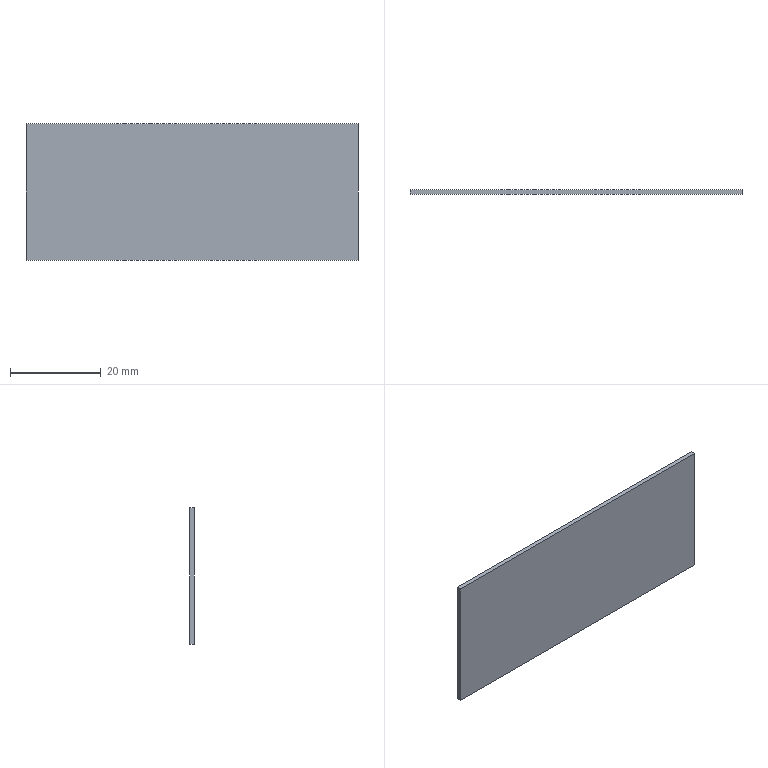Part | STEP file | 09-21 Inlet side seal plate | 1 solid | 6 faces | box 73 x 1 x 30 mm | volume 2190 mm3 | plane 6
STEP:
#1=CARTESIAN_POINT('',(0.,0.,0.));
#2=DIRECTION('',(0.,0.,1.));
#3=DIRECTION('',(1.,0.,0.));
#4=AXIS2_PLACEMENT_3D('',#1,#2,#3);
#5=CARTESIAN_POINT('',(73.,0.,0.));
#6=VERTEX_POINT('',#5);
#7=CARTESIAN_POINT('',(0.,0.,0.));
#8=VERTEX_POINT('',#7);
#9=CARTESIAN_POINT('',(36.5,0.,0.));
#10=DIRECTION('',(-1.,0.,0.));
#11=VECTOR('',#10,1.);
#12=LINE('',#9,#11);
#13=CARTESIAN_POINT('',(73.,0.,0.));
#14=DIRECTION('',(0.,0.,-1.));
#15=DIRECTION('',(-1.,0.,0.));
#16=AXIS2_PLACEMENT_3D('',#13,#14,#15);
#17=PLANE('',#16);
#18=CARTESIAN_POINT('',(36.5,0.));
#19=DIRECTION('',(1.,0.));
#20=VECTOR('',#19,1.);
#21=LINE('',#18,#20);
#22=(GEOMETRIC_REPRESENTATION_CONTEXT(2)PARAMETRIC_REPRESENTATION_CONTEXT()REPRESENTATION_CONTEXT('',''));
#23=DEFINITIONAL_REPRESENTATION('',(#21),#22);
#24=PCURVE('',#17,#23);
#25=CARTESIAN_POINT('',(0.,0.,-30.));
#26=DIRECTION('',(0.,1.,0.));
#27=DIRECTION('',(0.,0.,1.));
#28=AXIS2_PLACEMENT_3D('',#25,#26,#27);
#29=PLANE('',#28);
#30=CARTESIAN_POINT('',(30.,36.5));
#31=DIRECTION('',(0.,-1.));
#32=VECTOR('',#31,1.);
#33=LINE('',#30,#32);
#34=(GEOMETRIC_REPRESENTATION_CONTEXT(2)PARAMETRIC_REPRESENTATION_CONTEXT()REPRESENTATION_CONTEXT('',''));
#35=DEFINITIONAL_REPRESENTATION('',(#33),#34);
#36=PCURVE('',#29,#35);
#37=SURFACE_CURVE('',#12,(#24,#36),.PCURVE_S1.);
#38=EDGE_CURVE('',#6,#8,#37,.T.);
#39=ORIENTED_EDGE('',*,*,#38,.F.);
#40=CARTESIAN_POINT('',(73.,1.,0.));
#41=VERTEX_POINT('',#40);
#42=CARTESIAN_POINT('',(73.,0.5,0.));
#43=DIRECTION('',(0.,1.,0.));
#44=VECTOR('',#43,1.);
#45=LINE('',#42,#44);
#46=CARTESIAN_POINT('',(0.,0.5));
#47=DIRECTION('',(0.,1.));
#48=VECTOR('',#47,1.);
#49=LINE('',#46,#48);
#50=(GEOMETRIC_REPRESENTATION_CONTEXT(2)PARAMETRIC_REPRESENTATION_CONTEXT()REPRESENTATION_CONTEXT('',''));
#51=DEFINITIONAL_REPRESENTATION('',(#49),#50);
#52=PCURVE('',#17,#51);
#53=CARTESIAN_POINT('',(73.,0.,-30.));
#54=DIRECTION('',(-1.,0.,0.));
#55=DIRECTION('',(0.,0.,1.));
#56=AXIS2_PLACEMENT_3D('',#53,#54,#55);
#57=PLANE('',#56);
#58=CARTESIAN_POINT('',(30.,0.5));
#59=DIRECTION('',(0.,1.));
#60=VECTOR('',#59,1.);
#61=LINE('',#58,#60);
#62=(GEOMETRIC_REPRESENTATION_CONTEXT(2)PARAMETRIC_REPRESENTATION_CONTEXT()REPRESENTATION_CONTEXT('',''));
#63=DEFINITIONAL_REPRESENTATION('',(#61),#62);
#64=PCURVE('',#57,#63);
#65=SURFACE_CURVE('',#45,(#52,#64),.PCURVE_S1.);
#66=EDGE_CURVE('',#6,#41,#65,.T.);
#67=ORIENTED_EDGE('',*,*,#66,.T.);
#68=CARTESIAN_POINT('',(0.,1.,0.));
#69=VERTEX_POINT('',#68);
#70=CARTESIAN_POINT('',(36.5,1.,0.));
#71=DIRECTION('',(1.,0.,0.));
#72=VECTOR('',#71,1.);
#73=LINE('',#70,#72);
#74=CARTESIAN_POINT('',(36.5,1.));
#75=DIRECTION('',(-1.,0.));
#76=VECTOR('',#75,1.);
#77=LINE('',#74,#76);
#78=(GEOMETRIC_REPRESENTATION_CONTEXT(2)PARAMETRIC_REPRESENTATION_CONTEXT()REPRESENTATION_CONTEXT('',''));
#79=DEFINITIONAL_REPRESENTATION('',(#77),#78);
#80=PCURVE('',#17,#79);
#81=CARTESIAN_POINT('',(0.,1.,0.));
#82=DIRECTION('',(0.,-1.,0.));
#83=DIRECTION('',(0.,0.,-1.));
#84=AXIS2_PLACEMENT_3D('',#81,#82,#83);
#85=PLANE('',#84);
#86=CARTESIAN_POINT('',(0.,36.5));
#87=DIRECTION('',(0.,1.));
#88=VECTOR('',#87,1.);
#89=LINE('',#86,#88);
#90=(GEOMETRIC_REPRESENTATION_CONTEXT(2)PARAMETRIC_REPRESENTATION_CONTEXT()REPRESENTATION_CONTEXT('',''));
#91=DEFINITIONAL_REPRESENTATION('',(#89),#90);
#92=PCURVE('',#85,#91);
#93=SURFACE_CURVE('',#73,(#80,#92),.PCURVE_S1.);
#94=EDGE_CURVE('',#69,#41,#93,.T.);
#95=ORIENTED_EDGE('',*,*,#94,.F.);
#96=CARTESIAN_POINT('',(0.,0.5,0.));
#97=DIRECTION('',(0.,1.,0.));
#98=VECTOR('',#97,1.);
#99=LINE('',#96,#98);
#100=CARTESIAN_POINT('',(73.,0.5));
#101=DIRECTION('',(0.,1.));
#102=VECTOR('',#101,1.);
#103=LINE('',#100,#102);
#104=(GEOMETRIC_REPRESENTATION_CONTEXT(2)PARAMETRIC_REPRESENTATION_CONTEXT()REPRESENTATION_CONTEXT('',''));
#105=DEFINITIONAL_REPRESENTATION('',(#103),#104);
#106=PCURVE('',#17,#105);
#107=CARTESIAN_POINT('',(0.,0.,-30.));
#108=DIRECTION('',(-1.,0.,0.));
#109=DIRECTION('',(0.,0.,1.));
#110=AXIS2_PLACEMENT_3D('',#107,#108,#109);
#111=PLANE('',#110);
#112=CARTESIAN_POINT('',(30.,0.5));
#113=DIRECTION('',(0.,1.));
#114=VECTOR('',#113,1.);
#115=LINE('',#112,#114);
#116=(GEOMETRIC_REPRESENTATION_CONTEXT(2)PARAMETRIC_REPRESENTATION_CONTEXT()REPRESENTATION_CONTEXT('',''));
#117=DEFINITIONAL_REPRESENTATION('',(#115),#116);
#118=PCURVE('',#111,#117);
#119=SURFACE_CURVE('',#99,(#106,#118),.PCURVE_S1.);
#120=EDGE_CURVE('',#8,#69,#119,.T.);
#121=ORIENTED_EDGE('',*,*,#120,.F.);
#122=EDGE_LOOP('',(#39,#67,#95,#121));
#123=FACE_BOUND('',#122,.T.);
#124=ADVANCED_FACE('',(#123),#17,.F.);
#125=CARTESIAN_POINT('',(73.,0.,-30.));
#126=VERTEX_POINT('',#125);
#127=CARTESIAN_POINT('',(0.,0.,-30.));
#128=VERTEX_POINT('',#127);
#129=CARTESIAN_POINT('',(36.5,0.,-30.));
#130=DIRECTION('',(-1.,0.,0.));
#131=VECTOR('',#130,1.);
#132=LINE('',#129,#131);
#133=CARTESIAN_POINT('',(0.,36.5));
#134=DIRECTION('',(0.,-1.));
#135=VECTOR('',#134,1.);
#136=LINE('',#133,#135);
#137=(GEOMETRIC_REPRESENTATION_CONTEXT(2)PARAMETRIC_REPRESENTATION_CONTEXT()REPRESENTATION_CONTEXT('',''));
#138=DEFINITIONAL_REPRESENTATION('',(#136),#137);
#139=PCURVE('',#29,#138);
#140=CARTESIAN_POINT('',(0.,0.,-30.));
#141=DIRECTION('',(0.,0.,1.));
#142=DIRECTION('',(1.,0.,0.));
#143=AXIS2_PLACEMENT_3D('',#140,#141,#142);
#144=PLANE('',#143);
#145=CARTESIAN_POINT('',(36.5,0.));
#146=DIRECTION('',(-1.,0.));
#147=VECTOR('',#146,1.);
#148=LINE('',#145,#147);
#149=(GEOMETRIC_REPRESENTATION_CONTEXT(2)PARAMETRIC_REPRESENTATION_CONTEXT()REPRESENTATION_CONTEXT('',''));
#150=DEFINITIONAL_REPRESENTATION('',(#148),#149);
#151=PCURVE('',#144,#150);
#152=SURFACE_CURVE('',#132,(#139,#151),.PCURVE_S1.);
#153=EDGE_CURVE('',#126,#128,#152,.T.);
#154=ORIENTED_EDGE('',*,*,#153,.F.);
#155=CARTESIAN_POINT('',(73.,0.,-15.));
#156=DIRECTION('',(0.,0.,-1.));
#157=VECTOR('',#156,1.);
#158=LINE('',#155,#157);
#159=CARTESIAN_POINT('',(15.,73.));
#160=DIRECTION('',(-1.,0.));
#161=VECTOR('',#160,1.);
#162=LINE('',#159,#161);
#163=(GEOMETRIC_REPRESENTATION_CONTEXT(2)PARAMETRIC_REPRESENTATION_CONTEXT()REPRESENTATION_CONTEXT('',''));
#164=DEFINITIONAL_REPRESENTATION('',(#162),#163);
#165=PCURVE('',#29,#164);
#166=CARTESIAN_POINT('',(15.,0.));
#167=DIRECTION('',(-1.,0.));
#168=VECTOR('',#167,1.);
#169=LINE('',#166,#168);
#170=(GEOMETRIC_REPRESENTATION_CONTEXT(2)PARAMETRIC_REPRESENTATION_CONTEXT()REPRESENTATION_CONTEXT('',''));
#171=DEFINITIONAL_REPRESENTATION('',(#169),#170);
#172=PCURVE('',#57,#171);
#173=SURFACE_CURVE('',#158,(#165,#172),.PCURVE_S1.);
#174=EDGE_CURVE('',#6,#126,#173,.T.);
#175=ORIENTED_EDGE('',*,*,#174,.F.);
#176=ORIENTED_EDGE('',*,*,#38,.T.);
#177=CARTESIAN_POINT('',(0.,0.,-15.));
#178=DIRECTION('',(0.,0.,1.));
#179=VECTOR('',#178,1.);
#180=LINE('',#177,#179);
#181=CARTESIAN_POINT('',(15.,0.));
#182=DIRECTION('',(1.,0.));
#183=VECTOR('',#182,1.);
#184=LINE('',#181,#183);
#185=(GEOMETRIC_REPRESENTATION_CONTEXT(2)PARAMETRIC_REPRESENTATION_CONTEXT()REPRESENTATION_CONTEXT('',''));
#186=DEFINITIONAL_REPRESENTATION('',(#184),#185);
#187=PCURVE('',#29,#186);
#188=CARTESIAN_POINT('',(15.,0.));
#189=DIRECTION('',(1.,0.));
#190=VECTOR('',#189,1.);
#191=LINE('',#188,#190);
#192=(GEOMETRIC_REPRESENTATION_CONTEXT(2)PARAMETRIC_REPRESENTATION_CONTEXT()REPRESENTATION_CONTEXT('',''));
#193=DEFINITIONAL_REPRESENTATION('',(#191),#192);
#194=PCURVE('',#111,#193);
#195=SURFACE_CURVE('',#180,(#187,#194),.PCURVE_S1.);
#196=EDGE_CURVE('',#128,#8,#195,.T.);
#197=ORIENTED_EDGE('',*,*,#196,.F.);
#198=EDGE_LOOP('',(#154,#175,#176,#197));
#199=FACE_BOUND('',#198,.T.);
#200=ADVANCED_FACE('',(#199),#29,.F.);
#201=ORIENTED_EDGE('',*,*,#94,.T.);
#202=CARTESIAN_POINT('',(73.,1.,-30.));
#203=VERTEX_POINT('',#202);
#204=CARTESIAN_POINT('',(73.,1.,-15.));
#205=DIRECTION('',(0.,0.,1.));
#206=VECTOR('',#205,1.);
#207=LINE('',#204,#206);
#208=CARTESIAN_POINT('',(15.,73.));
#209=DIRECTION('',(-1.,0.));
#210=VECTOR('',#209,1.);
#211=LINE('',#208,#210);
#212=(GEOMETRIC_REPRESENTATION_CONTEXT(2)PARAMETRIC_REPRESENTATION_CONTEXT()REPRESENTATION_CONTEXT('',''));
#213=DEFINITIONAL_REPRESENTATION('',(#211),#212);
#214=PCURVE('',#85,#213);
#215=CARTESIAN_POINT('',(15.,1.));
#216=DIRECTION('',(1.,0.));
#217=VECTOR('',#216,1.);
#218=LINE('',#215,#217);
#219=(GEOMETRIC_REPRESENTATION_CONTEXT(2)PARAMETRIC_REPRESENTATION_CONTEXT()REPRESENTATION_CONTEXT('',''));
#220=DEFINITIONAL_REPRESENTATION('',(#218),#219);
#221=PCURVE('',#57,#220);
#222=SURFACE_CURVE('',#207,(#214,#221),.PCURVE_S1.);
#223=EDGE_CURVE('',#203,#41,#222,.T.);
#224=ORIENTED_EDGE('',*,*,#223,.F.);
#225=CARTESIAN_POINT('',(0.,1.,-30.));
#226=VERTEX_POINT('',#225);
#227=CARTESIAN_POINT('',(36.5,1.,-30.));
#228=DIRECTION('',(1.,0.,0.));
#229=VECTOR('',#228,1.);
#230=LINE('',#227,#229);
#231=CARTESIAN_POINT('',(30.,36.5));
#232=DIRECTION('',(0.,1.));
#233=VECTOR('',#232,1.);
#234=LINE('',#231,#233);
#235=(GEOMETRIC_REPRESENTATION_CONTEXT(2)PARAMETRIC_REPRESENTATION_CONTEXT()REPRESENTATION_CONTEXT('',''));
#236=DEFINITIONAL_REPRESENTATION('',(#234),#235);
#237=PCURVE('',#85,#236);
#238=CARTESIAN_POINT('',(36.5,1.));
#239=DIRECTION('',(1.,0.));
#240=VECTOR('',#239,1.);
#241=LINE('',#238,#240);
#242=(GEOMETRIC_REPRESENTATION_CONTEXT(2)PARAMETRIC_REPRESENTATION_CONTEXT()REPRESENTATION_CONTEXT('',''));
#243=DEFINITIONAL_REPRESENTATION('',(#241),#242);
#244=PCURVE('',#144,#243);
#245=SURFACE_CURVE('',#230,(#237,#244),.PCURVE_S1.);
#246=EDGE_CURVE('',#226,#203,#245,.T.);
#247=ORIENTED_EDGE('',*,*,#246,.F.);
#248=CARTESIAN_POINT('',(0.,1.,-15.));
#249=DIRECTION('',(0.,0.,-1.));
#250=VECTOR('',#249,1.);
#251=LINE('',#248,#250);
#252=CARTESIAN_POINT('',(15.,0.));
#253=DIRECTION('',(1.,0.));
#254=VECTOR('',#253,1.);
#255=LINE('',#252,#254);
#256=(GEOMETRIC_REPRESENTATION_CONTEXT(2)PARAMETRIC_REPRESENTATION_CONTEXT()REPRESENTATION_CONTEXT('',''));
#257=DEFINITIONAL_REPRESENTATION('',(#255),#256);
#258=PCURVE('',#85,#257);
#259=CARTESIAN_POINT('',(15.,1.));
#260=DIRECTION('',(-1.,0.));
#261=VECTOR('',#260,1.);
#262=LINE('',#259,#261);
#263=(GEOMETRIC_REPRESENTATION_CONTEXT(2)PARAMETRIC_REPRESENTATION_CONTEXT()REPRESENTATION_CONTEXT('',''));
#264=DEFINITIONAL_REPRESENTATION('',(#262),#263);
#265=PCURVE('',#111,#264);
#266=SURFACE_CURVE('',#251,(#258,#265),.PCURVE_S1.);
#267=EDGE_CURVE('',#69,#226,#266,.T.);
#268=ORIENTED_EDGE('',*,*,#267,.F.);
#269=EDGE_LOOP('',(#201,#224,#247,#268));
#270=FACE_BOUND('',#269,.T.);
#271=ADVANCED_FACE('',(#270),#85,.F.);
#272=CARTESIAN_POINT('',(0.,0.5,-30.));
#273=DIRECTION('',(0.,-1.,0.));
#274=VECTOR('',#273,1.);
#275=LINE('',#272,#274);
#276=CARTESIAN_POINT('',(0.,0.5));
#277=DIRECTION('',(0.,-1.));
#278=VECTOR('',#277,1.);
#279=LINE('',#276,#278);
#280=(GEOMETRIC_REPRESENTATION_CONTEXT(2)PARAMETRIC_REPRESENTATION_CONTEXT()REPRESENTATION_CONTEXT('',''));
#281=DEFINITIONAL_REPRESENTATION('',(#279),#280);
#282=PCURVE('',#111,#281);
#283=CARTESIAN_POINT('',(0.,0.5));
#284=DIRECTION('',(0.,-1.));
#285=VECTOR('',#284,1.);
#286=LINE('',#283,#285);
#287=(GEOMETRIC_REPRESENTATION_CONTEXT(2)PARAMETRIC_REPRESENTATION_CONTEXT()REPRESENTATION_CONTEXT('',''));
#288=DEFINITIONAL_REPRESENTATION('',(#286),#287);
#289=PCURVE('',#144,#288);
#290=SURFACE_CURVE('',#275,(#282,#289),.PCURVE_S1.);
#291=EDGE_CURVE('',#226,#128,#290,.T.);
#292=ORIENTED_EDGE('',*,*,#291,.T.);
#293=ORIENTED_EDGE('',*,*,#196,.T.);
#294=ORIENTED_EDGE('',*,*,#120,.T.);
#295=ORIENTED_EDGE('',*,*,#267,.T.);
#296=EDGE_LOOP('',(#292,#293,#294,#295));
#297=FACE_BOUND('',#296,.T.);
#298=ADVANCED_FACE('',(#297),#111,.T.);
#299=ORIENTED_EDGE('',*,*,#246,.T.);
#300=CARTESIAN_POINT('',(73.,0.5,-30.));
#301=DIRECTION('',(0.,1.,0.));
#302=VECTOR('',#301,1.);
#303=LINE('',#300,#302);
#304=CARTESIAN_POINT('',(73.,0.5));
#305=DIRECTION('',(0.,1.));
#306=VECTOR('',#305,1.);
#307=LINE('',#304,#306);
#308=(GEOMETRIC_REPRESENTATION_CONTEXT(2)PARAMETRIC_REPRESENTATION_CONTEXT()REPRESENTATION_CONTEXT('',''));
#309=DEFINITIONAL_REPRESENTATION('',(#307),#308);
#310=PCURVE('',#144,#309);
#311=CARTESIAN_POINT('',(0.,0.5));
#312=DIRECTION('',(0.,1.));
#313=VECTOR('',#312,1.);
#314=LINE('',#311,#313);
#315=(GEOMETRIC_REPRESENTATION_CONTEXT(2)PARAMETRIC_REPRESENTATION_CONTEXT()REPRESENTATION_CONTEXT('',''));
#316=DEFINITIONAL_REPRESENTATION('',(#314),#315);
#317=PCURVE('',#57,#316);
#318=SURFACE_CURVE('',#303,(#310,#317),.PCURVE_S1.);
#319=EDGE_CURVE('',#126,#203,#318,.T.);
#320=ORIENTED_EDGE('',*,*,#319,.F.);
#321=ORIENTED_EDGE('',*,*,#153,.T.);
#322=ORIENTED_EDGE('',*,*,#291,.F.);
#323=EDGE_LOOP('',(#299,#320,#321,#322));
#324=FACE_BOUND('',#323,.T.);
#325=ADVANCED_FACE('',(#324),#144,.F.);
#326=ORIENTED_EDGE('',*,*,#174,.T.);
#327=ORIENTED_EDGE('',*,*,#319,.T.);
#328=ORIENTED_EDGE('',*,*,#223,.T.);
#329=ORIENTED_EDGE('',*,*,#66,.F.);
#330=EDGE_LOOP('',(#326,#327,#328,#329));
#331=FACE_BOUND('',#330,.T.);
#332=ADVANCED_FACE('',(#331),#57,.F.);
#333=CLOSED_SHELL('',(#124,#200,#271,#298,#325,#332));
#334=MANIFOLD_SOLID_BREP('',#333);
#335=(LENGTH_UNIT()NAMED_UNIT(*)SI_UNIT(.MILLI.,.METRE.));
#336=UNCERTAINTY_MEASURE_WITH_UNIT(LENGTH_MEASURE(0.0000001),#335,'','');
#337=(NAMED_UNIT(*)PLANE_ANGLE_UNIT()SI_UNIT($,.RADIAN.));
#338=(NAMED_UNIT(*)SI_UNIT($,.STERADIAN.)SOLID_ANGLE_UNIT());
#339=(GEOMETRIC_REPRESENTATION_CONTEXT(3)GLOBAL_UNCERTAINTY_ASSIGNED_CONTEXT((#336))GLOBAL_UNIT_ASSIGNED_CONTEXT((#335,#337,#338))REPRESENTATION_CONTEXT('',''));
#340=ADVANCED_BREP_SHAPE_REPRESENTATION('',(#4,#334),#339);